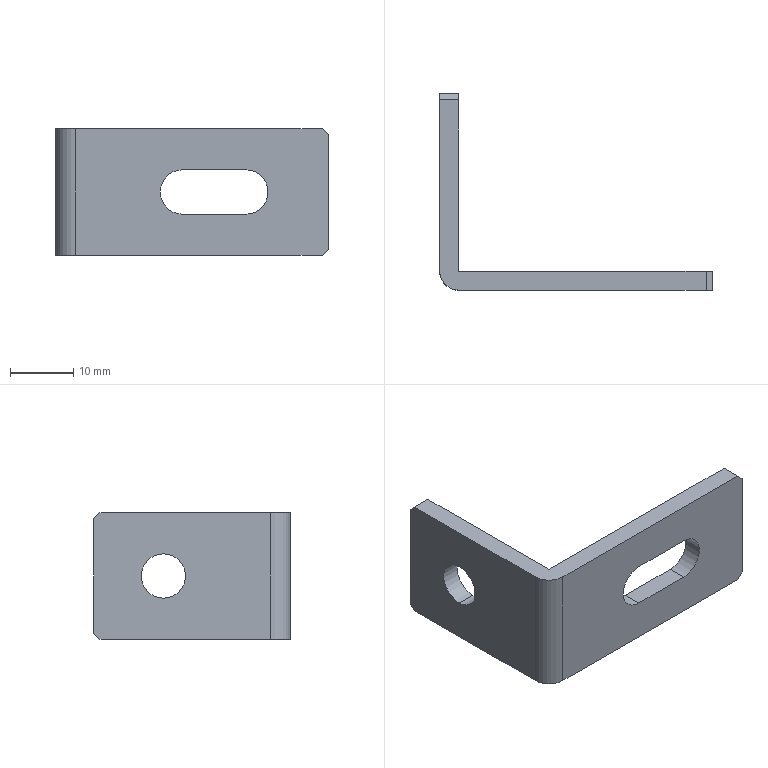Part | SolidWorks | features BaseBody 1 | 1 solid | 21 faces | box 43 x 31 x 20 mm | volume 3772 mm3 | plane 14 | cylinder 7 | commonest cylinder face diameters 7 x5 0.2 x1 6.2 x1
STEP:
#1=CARTESIAN_POINT('',(16.5,-31.,10.));
#2=VERTEX_POINT('',#1);
#3=CARTESIAN_POINT('',(20.,-31.,13.5));
#4=VERTEX_POINT('',#3);
#5=CARTESIAN_POINT('',(20.,-31.,10.));
#6=DIRECTION('',(0.,1.,0.));
#7=DIRECTION('',(-1.,0.,0.));
#8=AXIS2_PLACEMENT_3D('',#5,#6,#7);
#9=CIRCLE('',#8,3.5);
#10=EDGE_CURVE('',#2,#4,#9,.T.);
#11=ORIENTED_EDGE('',*,*,#10,.F.);
#12=CARTESIAN_POINT('',(16.5,-28.,10.));
#13=VERTEX_POINT('',#12);
#14=CARTESIAN_POINT('',(16.5,-31.,10.));
#15=DIRECTION('',(0.,1.,0.));
#16=VECTOR('',#15,1000.);
#17=LINE('',#14,#16);
#18=EDGE_CURVE('',#2,#13,#17,.T.);
#19=ORIENTED_EDGE('',*,*,#18,.T.);
#20=CARTESIAN_POINT('',(20.,-28.,13.5));
#21=VERTEX_POINT('',#20);
#22=CARTESIAN_POINT('',(20.,-28.,10.));
#23=DIRECTION('',(0.,1.,0.));
#24=DIRECTION('',(-1.,0.,0.));
#25=AXIS2_PLACEMENT_3D('',#22,#23,#24);
#26=CIRCLE('',#25,3.5);
#27=EDGE_CURVE('',#13,#21,#26,.T.);
#28=ORIENTED_EDGE('',*,*,#27,.T.);
#29=CARTESIAN_POINT('',(20.,-31.,13.5));
#30=DIRECTION('',(0.,-1.,0.));
#31=VECTOR('',#30,1000.);
#32=LINE('',#29,#31);
#33=EDGE_CURVE('',#21,#4,#32,.T.);
#34=ORIENTED_EDGE('',*,*,#33,.T.);
#35=EDGE_LOOP('',(#11,#19,#28,#34));
#36=FACE_OUTER_BOUND('',#35,.T.);
#37=CARTESIAN_POINT('',(20.,-31.,10.));
#38=DIRECTION('',(0.,1.,0.));
#39=DIRECTION('',(-1.,0.,0.));
#40=AXIS2_PLACEMENT_3D('',#37,#38,#39);
#41=CYLINDRICAL_SURFACE('',#40,3.5);
#42=ADVANCED_FACE('',(#36),#41,.F.);
#43=CARTESIAN_POINT('',(0.,-11.,13.5));
#44=VERTEX_POINT('',#43);
#45=CARTESIAN_POINT('',(0.,-11.,6.5));
#46=VERTEX_POINT('',#45);
#47=CARTESIAN_POINT('',(0.,-11.,10.));
#48=DIRECTION('',(1.,0.,0.));
#49=DIRECTION('',(0.,0.,-1.));
#50=AXIS2_PLACEMENT_3D('',#47,#48,#49);
#51=CIRCLE('',#50,3.5);
#52=EDGE_CURVE('',#44,#46,#51,.T.);
#53=ORIENTED_EDGE('',*,*,#52,.F.);
#54=CARTESIAN_POINT('',(3.,-11.,13.5));
#55=VERTEX_POINT('',#54);
#56=CARTESIAN_POINT('',(3.,-11.,13.5));
#57=DIRECTION('',(1.,0.,0.));
#58=VECTOR('',#57,1000.);
#59=LINE('',#56,#58);
#60=EDGE_CURVE('',#44,#55,#59,.T.);
#61=ORIENTED_EDGE('',*,*,#60,.T.);
#62=CARTESIAN_POINT('',(3.,-11.,6.5));
#63=VERTEX_POINT('',#62);
#64=CARTESIAN_POINT('',(3.,-11.,10.));
#65=DIRECTION('',(1.,0.,0.));
#66=DIRECTION('',(0.,0.,-1.));
#67=AXIS2_PLACEMENT_3D('',#64,#65,#66);
#68=CIRCLE('',#67,3.5);
#69=EDGE_CURVE('',#55,#63,#68,.T.);
#70=ORIENTED_EDGE('',*,*,#69,.T.);
#71=CARTESIAN_POINT('',(3.,-11.,6.5));
#72=DIRECTION('',(1.,0.,0.));
#73=VECTOR('',#72,1000.);
#74=LINE('',#71,#73);
#75=EDGE_CURVE('',#46,#63,#74,.T.);
#76=ORIENTED_EDGE('',*,*,#75,.F.);
#77=EDGE_LOOP('',(#53,#61,#70,#76));
#78=FACE_OUTER_BOUND('',#77,.T.);
#79=CARTESIAN_POINT('',(3.,-11.,10.));
#80=DIRECTION('',(1.,0.,0.));
#81=DIRECTION('',(0.,0.,-1.));
#82=AXIS2_PLACEMENT_3D('',#79,#80,#81);
#83=CYLINDRICAL_SURFACE('',#82,3.5);
#84=ADVANCED_FACE('',(#78),#83,.F.);
#85=CARTESIAN_POINT('',(43.,-28.,1.));
#86=VERTEX_POINT('',#85);
#87=CARTESIAN_POINT('',(42.,-28.,0.));
#88=VERTEX_POINT('',#87);
#89=CARTESIAN_POINT('',(42.,-28.,0.));
#90=DIRECTION('',(-0.7071,0.,-0.7071));
#91=VECTOR('',#90,1000.);
#92=LINE('',#89,#91);
#93=EDGE_CURVE('',#86,#88,#92,.T.);
#94=ORIENTED_EDGE('',*,*,#93,.T.);
#95=CARTESIAN_POINT('',(3.1,-28.,0.));
#96=VERTEX_POINT('',#95);
#97=CARTESIAN_POINT('',(43.,-28.,0.));
#98=DIRECTION('',(1.,0.,0.));
#99=VECTOR('',#98,1000.);
#100=LINE('',#97,#99);
#101=EDGE_CURVE('',#96,#88,#100,.T.);
#102=ORIENTED_EDGE('',*,*,#101,.F.);
#103=CARTESIAN_POINT('',(3.1,-28.,20.));
#104=VERTEX_POINT('',#103);
#105=CARTESIAN_POINT('',(3.1,-28.,20.));
#106=DIRECTION('',(0.,0.,-1.));
#107=VECTOR('',#106,1000.);
#108=LINE('',#105,#107);
#109=EDGE_CURVE('',#104,#96,#108,.T.);
#110=ORIENTED_EDGE('',*,*,#109,.F.);
#111=CARTESIAN_POINT('',(42.,-28.,20.));
#112=VERTEX_POINT('',#111);
#113=CARTESIAN_POINT('',(43.,-28.,20.));
#114=DIRECTION('',(-1.,0.,0.));
#115=VECTOR('',#114,1000.);
#116=LINE('',#113,#115);
#117=EDGE_CURVE('',#112,#104,#116,.T.);
#118=ORIENTED_EDGE('',*,*,#117,.F.);
#119=CARTESIAN_POINT('',(43.,-28.,19.));
#120=VERTEX_POINT('',#119);
#121=CARTESIAN_POINT('',(43.,-28.,19.));
#122=DIRECTION('',(-0.7071,0.,0.7071));
#123=VECTOR('',#122,1000.);
#124=LINE('',#121,#123);
#125=EDGE_CURVE('',#120,#112,#124,.T.);
#126=ORIENTED_EDGE('',*,*,#125,.F.);
#127=CARTESIAN_POINT('',(43.,-28.,20.));
#128=DIRECTION('',(0.,0.,1.));
#129=VECTOR('',#128,1000.);
#130=LINE('',#127,#129);
#131=EDGE_CURVE('',#86,#120,#130,.T.);
#132=ORIENTED_EDGE('',*,*,#131,.F.);
#133=EDGE_LOOP('',(#94,#102,#110,#118,#126,#132));
#134=FACE_OUTER_BOUND('',#133,.T.);
#135=CARTESIAN_POINT('',(30.,-28.,13.5));
#136=VERTEX_POINT('',#135);
#137=CARTESIAN_POINT('',(43.,-28.,13.5));
#138=DIRECTION('',(1.,0.,0.));
#139=VECTOR('',#138,1000.);
#140=LINE('',#137,#139);
#141=EDGE_CURVE('',#21,#136,#140,.T.);
#142=ORIENTED_EDGE('',*,*,#141,.F.);
#143=ORIENTED_EDGE('',*,*,#27,.F.);
#144=CARTESIAN_POINT('',(20.,-28.,6.5));
#145=VERTEX_POINT('',#144);
#146=CARTESIAN_POINT('',(20.,-28.,10.));
#147=DIRECTION('',(0.,1.,0.));
#148=DIRECTION('',(-1.,0.,0.));
#149=AXIS2_PLACEMENT_3D('',#146,#147,#148);
#150=CIRCLE('',#149,3.5);
#151=EDGE_CURVE('',#145,#13,#150,.T.);
#152=ORIENTED_EDGE('',*,*,#151,.F.);
#153=CARTESIAN_POINT('',(30.,-28.,6.5));
#154=VERTEX_POINT('',#153);
#155=CARTESIAN_POINT('',(43.,-28.,6.5));
#156=DIRECTION('',(-1.,0.,0.));
#157=VECTOR('',#156,1000.);
#158=LINE('',#155,#157);
#159=EDGE_CURVE('',#154,#145,#158,.T.);
#160=ORIENTED_EDGE('',*,*,#159,.F.);
#161=CARTESIAN_POINT('',(30.,-28.,10.));
#162=DIRECTION('',(0.,1.,0.));
#163=DIRECTION('',(-1.,0.,0.));
#164=AXIS2_PLACEMENT_3D('',#161,#162,#163);
#165=CIRCLE('',#164,3.5);
#166=EDGE_CURVE('',#136,#154,#165,.T.);
#167=ORIENTED_EDGE('',*,*,#166,.F.);
#168=EDGE_LOOP('',(#142,#143,#152,#160,#167));
#169=FACE_BOUND('',#168,.T.);
#170=CARTESIAN_POINT('',(43.,-28.,20.));
#171=DIRECTION('',(0.,-1.,0.));
#172=DIRECTION('',(1.,0.,0.));
#173=AXIS2_PLACEMENT_3D('',#170,#171,#172);
#174=PLANE('',#173);
#175=ADVANCED_FACE('',(#134,#169),#174,.F.);
#176=ORIENTED_EDGE('',*,*,#131,.T.);
#177=CARTESIAN_POINT('',(43.,-31.,19.));
#178=VERTEX_POINT('',#177);
#179=CARTESIAN_POINT('',(43.,-28.,19.));
#180=DIRECTION('',(0.,-1.,0.));
#181=VECTOR('',#180,1000.);
#182=LINE('',#179,#181);
#183=EDGE_CURVE('',#120,#178,#182,.T.);
#184=ORIENTED_EDGE('',*,*,#183,.T.);
#185=CARTESIAN_POINT('',(43.,-31.,1.));
#186=VERTEX_POINT('',#185);
#187=CARTESIAN_POINT('',(43.,-31.,20.));
#188=DIRECTION('',(0.,0.,-1.));
#189=VECTOR('',#188,1000.);
#190=LINE('',#187,#189);
#191=EDGE_CURVE('',#178,#186,#190,.T.);
#192=ORIENTED_EDGE('',*,*,#191,.T.);
#193=CARTESIAN_POINT('',(43.,-28.,1.));
#194=DIRECTION('',(0.,1.,0.));
#195=VECTOR('',#194,1000.);
#196=LINE('',#193,#195);
#197=EDGE_CURVE('',#186,#86,#196,.T.);
#198=ORIENTED_EDGE('',*,*,#197,.T.);
#199=EDGE_LOOP('',(#176,#184,#192,#198));
#200=FACE_OUTER_BOUND('',#199,.T.);
#201=CARTESIAN_POINT('',(43.,-28.,20.));
#202=DIRECTION('',(1.,0.,0.));
#203=DIRECTION('',(0.,0.,-1.));
#204=AXIS2_PLACEMENT_3D('',#201,#202,#203);
#205=PLANE('',#204);
#206=ADVANCED_FACE('',(#200),#205,.T.);
#207=CARTESIAN_POINT('',(42.,-31.,0.));
#208=VERTEX_POINT('',#207);
#209=CARTESIAN_POINT('',(3.1,-31.,0.));
#210=VERTEX_POINT('',#209);
#211=CARTESIAN_POINT('',(3.,-31.,0.));
#212=DIRECTION('',(-1.,0.,0.));
#213=VECTOR('',#212,1000.);
#214=LINE('',#211,#213);
#215=EDGE_CURVE('',#208,#210,#214,.T.);
#216=ORIENTED_EDGE('',*,*,#215,.T.);
#217=CARTESIAN_POINT('',(0.,-27.9,0.));
#218=VERTEX_POINT('',#217);
#219=CARTESIAN_POINT('',(3.1,-27.9,0.));
#220=DIRECTION('',(0.,0.,-1.));
#221=DIRECTION('',(-1.,0.,0.));
#222=AXIS2_PLACEMENT_3D('',#219,#220,#221);
#223=CIRCLE('',#222,3.1);
#224=EDGE_CURVE('',#210,#218,#223,.T.);
#225=ORIENTED_EDGE('',*,*,#224,.T.);
#226=CARTESIAN_POINT('',(0.,-1.,0.));
#227=VERTEX_POINT('',#226);
#228=CARTESIAN_POINT('',(0.,-27.9,0.));
#229=DIRECTION('',(0.,1.,0.));
#230=VECTOR('',#229,1000.);
#231=LINE('',#228,#230);
#232=EDGE_CURVE('',#218,#227,#231,.T.);
#233=ORIENTED_EDGE('',*,*,#232,.T.);
#234=CARTESIAN_POINT('',(3.,-1.,0.));
#235=VERTEX_POINT('',#234);
#236=CARTESIAN_POINT('',(3.1,-1.,0.));
#237=DIRECTION('',(1.,0.,0.));
#238=VECTOR('',#237,1000.);
#239=LINE('',#236,#238);
#240=EDGE_CURVE('',#227,#235,#239,.T.);
#241=ORIENTED_EDGE('',*,*,#240,.T.);
#242=CARTESIAN_POINT('',(3.,-27.9,0.));
#243=VERTEX_POINT('',#242);
#244=CARTESIAN_POINT('',(3.,0.,0.));
#245=DIRECTION('',(0.,-1.,0.));
#246=VECTOR('',#245,1000.);
#247=LINE('',#244,#246);
#248=EDGE_CURVE('',#235,#243,#247,.T.);
#249=ORIENTED_EDGE('',*,*,#248,.T.);
#250=CARTESIAN_POINT('',(3.1,-27.9,0.));
#251=DIRECTION('',(0.,0.,1.));
#252=DIRECTION('',(-1.,0.,0.));
#253=AXIS2_PLACEMENT_3D('',#250,#251,#252);
#254=CIRCLE('',#253,0.1);
#255=EDGE_CURVE('',#243,#96,#254,.T.);
#256=ORIENTED_EDGE('',*,*,#255,.T.);
#257=ORIENTED_EDGE('',*,*,#101,.T.);
#258=CARTESIAN_POINT('',(42.,-27.9,0.));
#259=DIRECTION('',(0.,-1.,0.));
#260=VECTOR('',#259,1000.);
#261=LINE('',#258,#260);
#262=EDGE_CURVE('',#88,#208,#261,.T.);
#263=ORIENTED_EDGE('',*,*,#262,.T.);
#264=EDGE_LOOP('',(#216,#225,#233,#241,#249,#256,#257,#263));
#265=FACE_OUTER_BOUND('',#264,.T.);
#266=CARTESIAN_POINT('',(3.,-27.9,0.));
#267=DIRECTION('',(0.,0.,-1.));
#268=DIRECTION('',(-1.,0.,0.));
#269=AXIS2_PLACEMENT_3D('',#266,#267,#268);
#270=PLANE('',#269);
#271=ADVANCED_FACE('',(#265),#270,.T.);
#272=CARTESIAN_POINT('',(3.,-27.9,20.));
#273=VERTEX_POINT('',#272);
#274=CARTESIAN_POINT('',(3.,-27.9,20.));
#275=DIRECTION('',(0.,0.,-1.));
#276=VECTOR('',#275,1000.);
#277=LINE('',#274,#276);
#278=EDGE_CURVE('',#273,#243,#277,.T.);
#279=ORIENTED_EDGE('',*,*,#278,.F.);
#280=CARTESIAN_POINT('',(3.1,-27.9,20.));
#281=DIRECTION('',(0.,0.,-1.));
#282=DIRECTION('',(-1.,0.,0.));
#283=AXIS2_PLACEMENT_3D('',#280,#281,#282);
#284=CIRCLE('',#283,0.1);
#285=EDGE_CURVE('',#104,#273,#284,.T.);
#286=ORIENTED_EDGE('',*,*,#285,.F.);
#287=ORIENTED_EDGE('',*,*,#109,.T.);
#288=ORIENTED_EDGE('',*,*,#255,.F.);
#289=EDGE_LOOP('',(#279,#286,#287,#288));
#290=FACE_OUTER_BOUND('',#289,.T.);
#291=CARTESIAN_POINT('',(3.1,-27.9,20.));
#292=DIRECTION('',(0.,0.,-1.));
#293=DIRECTION('',(-1.,0.,0.));
#294=AXIS2_PLACEMENT_3D('',#291,#292,#293);
#295=CYLINDRICAL_SURFACE('',#294,0.1);
#296=ADVANCED_FACE('',(#290),#295,.F.);
#297=CARTESIAN_POINT('',(42.,-31.,20.));
#298=VERTEX_POINT('',#297);
#299=CARTESIAN_POINT('',(42.,-27.9,20.));
#300=DIRECTION('',(0.,-1.,0.));
#301=VECTOR('',#300,1000.);
#302=LINE('',#299,#301);
#303=EDGE_CURVE('',#112,#298,#302,.T.);
#304=ORIENTED_EDGE('',*,*,#303,.F.);
#305=ORIENTED_EDGE('',*,*,#117,.T.);
#306=ORIENTED_EDGE('',*,*,#285,.T.);
#307=CARTESIAN_POINT('',(3.,-1.,20.));
#308=VERTEX_POINT('',#307);
#309=CARTESIAN_POINT('',(3.,0.,20.));
#310=DIRECTION('',(0.,1.,0.));
#311=VECTOR('',#310,1000.);
#312=LINE('',#309,#311);
#313=EDGE_CURVE('',#273,#308,#312,.T.);
#314=ORIENTED_EDGE('',*,*,#313,.T.);
#315=CARTESIAN_POINT('',(0.,-1.,20.));
#316=VERTEX_POINT('',#315);
#317=CARTESIAN_POINT('',(3.1,-1.,20.));
#318=DIRECTION('',(-1.,0.,0.));
#319=VECTOR('',#318,1000.);
#320=LINE('',#317,#319);
#321=EDGE_CURVE('',#308,#316,#320,.T.);
#322=ORIENTED_EDGE('',*,*,#321,.T.);
#323=CARTESIAN_POINT('',(0.,-27.9,20.));
#324=VERTEX_POINT('',#323);
#325=CARTESIAN_POINT('',(0.,-28.,20.));
#326=DIRECTION('',(0.,-1.,0.));
#327=VECTOR('',#326,1000.);
#328=LINE('',#325,#327);
#329=EDGE_CURVE('',#316,#324,#328,.T.);
#330=ORIENTED_EDGE('',*,*,#329,.T.);
#331=CARTESIAN_POINT('',(3.1,-31.,20.));
#332=VERTEX_POINT('',#331);
#333=CARTESIAN_POINT('',(3.1,-27.9,20.));
#334=DIRECTION('',(0.,0.,1.));
#335=DIRECTION('',(-1.,0.,0.));
#336=AXIS2_PLACEMENT_3D('',#333,#334,#335);
#337=CIRCLE('',#336,3.1);
#338=EDGE_CURVE('',#324,#332,#337,.T.);
#339=ORIENTED_EDGE('',*,*,#338,.T.);
#340=CARTESIAN_POINT('',(3.1,-31.,20.));
#341=DIRECTION('',(-1.,0.,0.));
#342=VECTOR('',#341,1000.);
#343=LINE('',#340,#342);
#344=EDGE_CURVE('',#298,#332,#343,.T.);
#345=ORIENTED_EDGE('',*,*,#344,.F.);
#346=EDGE_LOOP('',(#304,#305,#306,#314,#322,#330,#339,#345));
#347=FACE_OUTER_BOUND('',#346,.T.);
#348=CARTESIAN_POINT('',(3.1,-27.9,20.));
#349=DIRECTION('',(0.,0.,-1.));
#350=DIRECTION('',(-1.,0.,0.));
#351=AXIS2_PLACEMENT_3D('',#348,#349,#350);
#352=PLANE('',#351);
#353=ADVANCED_FACE('',(#347),#352,.F.);
#354=CARTESIAN_POINT('',(30.,-31.,13.5));
#355=VERTEX_POINT('',#354);
#356=CARTESIAN_POINT('',(30.,-31.,13.5));
#357=DIRECTION('',(0.,1.,0.));
#358=VECTOR('',#357,1000.);
#359=LINE('',#356,#358);
#360=EDGE_CURVE('',#355,#136,#359,.T.);
#361=ORIENTED_EDGE('',*,*,#360,.F.);
#362=CARTESIAN_POINT('',(20.,-31.,13.5));
#363=DIRECTION('',(1.,0.,0.));
#364=VECTOR('',#363,1000.);
#365=LINE('',#362,#364);
#366=EDGE_CURVE('',#4,#355,#365,.T.);
#367=ORIENTED_EDGE('',*,*,#366,.F.);
#368=ORIENTED_EDGE('',*,*,#33,.F.);
#369=ORIENTED_EDGE('',*,*,#141,.T.);
#370=EDGE_LOOP('',(#361,#367,#368,#369));
#371=FACE_OUTER_BOUND('',#370,.T.);
#372=CARTESIAN_POINT('',(20.,-31.,13.5));
#373=DIRECTION('',(0.,0.,1.));
#374=DIRECTION('',(1.,0.,0.));
#375=AXIS2_PLACEMENT_3D('',#372,#373,#374);
#376=PLANE('',#375);
#377=ADVANCED_FACE('',(#371),#376,.F.);
#378=ORIENTED_EDGE('',*,*,#18,.F.);
#379=CARTESIAN_POINT('',(20.,-31.,6.5));
#380=VERTEX_POINT('',#379);
#381=CARTESIAN_POINT('',(20.,-31.,10.));
#382=DIRECTION('',(0.,1.,0.));
#383=DIRECTION('',(-1.,0.,0.));
#384=AXIS2_PLACEMENT_3D('',#381,#382,#383);
#385=CIRCLE('',#384,3.5);
#386=EDGE_CURVE('',#380,#2,#385,.T.);
#387=ORIENTED_EDGE('',*,*,#386,.F.);
#388=CARTESIAN_POINT('',(20.,-31.,6.5));
#389=DIRECTION('',(0.,-1.,0.));
#390=VECTOR('',#389,1000.);
#391=LINE('',#388,#390);
#392=EDGE_CURVE('',#145,#380,#391,.T.);
#393=ORIENTED_EDGE('',*,*,#392,.F.);
#394=ORIENTED_EDGE('',*,*,#151,.T.);
#395=EDGE_LOOP('',(#378,#387,#393,#394));
#396=FACE_OUTER_BOUND('',#395,.T.);
#397=CARTESIAN_POINT('',(20.,-31.,10.));
#398=DIRECTION('',(0.,1.,0.));
#399=DIRECTION('',(-1.,0.,0.));
#400=AXIS2_PLACEMENT_3D('',#397,#398,#399);
#401=CYLINDRICAL_SURFACE('',#400,3.5);
#402=ADVANCED_FACE('',(#396),#401,.F.);
#403=ORIENTED_EDGE('',*,*,#392,.T.);
#404=CARTESIAN_POINT('',(30.,-31.,6.5));
#405=VERTEX_POINT('',#404);
#406=CARTESIAN_POINT('',(20.,-31.,6.5));
#407=DIRECTION('',(-1.,0.,0.));
#408=VECTOR('',#407,1000.);
#409=LINE('',#406,#408);
#410=EDGE_CURVE('',#405,#380,#409,.T.);
#411=ORIENTED_EDGE('',*,*,#410,.F.);
#412=CARTESIAN_POINT('',(30.,-31.,6.5));
#413=DIRECTION('',(0.,-1.,0.));
#414=VECTOR('',#413,1000.);
#415=LINE('',#412,#414);
#416=EDGE_CURVE('',#154,#405,#415,.T.);
#417=ORIENTED_EDGE('',*,*,#416,.F.);
#418=ORIENTED_EDGE('',*,*,#159,.T.);
#419=EDGE_LOOP('',(#403,#411,#417,#418));
#420=FACE_OUTER_BOUND('',#419,.T.);
#421=CARTESIAN_POINT('',(20.,-31.,6.5));
#422=DIRECTION('',(0.,0.,-1.));
#423=DIRECTION('',(-1.,0.,0.));
#424=AXIS2_PLACEMENT_3D('',#421,#422,#423);
#425=PLANE('',#424);
#426=ADVANCED_FACE('',(#420),#425,.F.);
#427=ORIENTED_EDGE('',*,*,#416,.T.);
#428=CARTESIAN_POINT('',(30.,-31.,10.));
#429=DIRECTION('',(0.,1.,0.));
#430=DIRECTION('',(-1.,0.,0.));
#431=AXIS2_PLACEMENT_3D('',#428,#429,#430);
#432=CIRCLE('',#431,3.5);
#433=EDGE_CURVE('',#355,#405,#432,.T.);
#434=ORIENTED_EDGE('',*,*,#433,.F.);
#435=ORIENTED_EDGE('',*,*,#360,.T.);
#436=ORIENTED_EDGE('',*,*,#166,.T.);
#437=EDGE_LOOP('',(#427,#434,#435,#436));
#438=FACE_OUTER_BOUND('',#437,.T.);
#439=CARTESIAN_POINT('',(30.,-31.,10.));
#440=DIRECTION('',(0.,1.,0.));
#441=DIRECTION('',(-1.,0.,0.));
#442=AXIS2_PLACEMENT_3D('',#439,#440,#441);
#443=CYLINDRICAL_SURFACE('',#442,3.5);
#444=ADVANCED_FACE('',(#438),#443,.F.);
#445=CARTESIAN_POINT('',(43.,-31.,19.));
#446=DIRECTION('',(0.7071,0.,-0.7071));
#447=VECTOR('',#446,1000.);
#448=LINE('',#445,#447);
#449=EDGE_CURVE('',#298,#178,#448,.T.);
#450=ORIENTED_EDGE('',*,*,#449,.T.);
#451=ORIENTED_EDGE('',*,*,#183,.F.);
#452=ORIENTED_EDGE('',*,*,#125,.T.);
#453=ORIENTED_EDGE('',*,*,#303,.T.);
#454=EDGE_LOOP('',(#450,#451,#452,#453));
#455=FACE_OUTER_BOUND('',#454,.T.);
#456=CARTESIAN_POINT('',(43.,-28.,19.));
#457=DIRECTION('',(0.7071,0.,0.7071));
#458=DIRECTION('',(0.7071,0.,-0.7071));
#459=AXIS2_PLACEMENT_3D('',#456,#457,#458);
#460=PLANE('',#459);
#461=ADVANCED_FACE('',(#455),#460,.T.);
#462=ORIENTED_EDGE('',*,*,#197,.F.);
#463=CARTESIAN_POINT('',(42.,-31.,0.));
#464=DIRECTION('',(0.7071,0.,0.7071));
#465=VECTOR('',#464,1000.);
#466=LINE('',#463,#465);
#467=EDGE_CURVE('',#208,#186,#466,.T.);
#468=ORIENTED_EDGE('',*,*,#467,.F.);
#469=ORIENTED_EDGE('',*,*,#262,.F.);
#470=ORIENTED_EDGE('',*,*,#93,.F.);
#471=EDGE_LOOP('',(#462,#468,#469,#470));
#472=FACE_OUTER_BOUND('',#471,.T.);
#473=CARTESIAN_POINT('',(42.,-27.9,0.));
#474=DIRECTION('',(-0.7071,0.,0.7071));
#475=DIRECTION('',(0.7071,0.,0.7071));
#476=AXIS2_PLACEMENT_3D('',#473,#474,#475);
#477=PLANE('',#476);
#478=ADVANCED_FACE('',(#472),#477,.F.);
#479=ORIENTED_EDGE('',*,*,#344,.T.);
#480=CARTESIAN_POINT('',(3.1,-31.,20.));
#481=DIRECTION('',(0.,0.,-1.));
#482=VECTOR('',#481,1000.);
#483=LINE('',#480,#482);
#484=EDGE_CURVE('',#332,#210,#483,.T.);
#485=ORIENTED_EDGE('',*,*,#484,.T.);
#486=ORIENTED_EDGE('',*,*,#215,.F.);
#487=ORIENTED_EDGE('',*,*,#467,.T.);
#488=ORIENTED_EDGE('',*,*,#191,.F.);
#489=ORIENTED_EDGE('',*,*,#449,.F.);
#490=EDGE_LOOP('',(#479,#485,#486,#487,#488,#489));
#491=FACE_OUTER_BOUND('',#490,.T.);
#492=ORIENTED_EDGE('',*,*,#433,.T.);
#493=ORIENTED_EDGE('',*,*,#410,.T.);
#494=ORIENTED_EDGE('',*,*,#386,.T.);
#495=ORIENTED_EDGE('',*,*,#10,.T.);
#496=ORIENTED_EDGE('',*,*,#366,.T.);
#497=EDGE_LOOP('',(#492,#493,#494,#495,#496));
#498=FACE_BOUND('',#497,.T.);
#499=CARTESIAN_POINT('',(43.,-31.,20.));
#500=DIRECTION('',(0.,-1.,0.));
#501=DIRECTION('',(1.,0.,0.));
#502=AXIS2_PLACEMENT_3D('',#499,#500,#501);
#503=PLANE('',#502);
#504=ADVANCED_FACE('',(#491,#498),#503,.T.);
#505=CARTESIAN_POINT('',(3.,0.,1.));
#506=VERTEX_POINT('',#505);
#507=CARTESIAN_POINT('',(3.,-1.,0.));
#508=DIRECTION('',(0.,0.7071,0.7071));
#509=VECTOR('',#508,1000.);
#510=LINE('',#507,#509);
#511=EDGE_CURVE('',#235,#506,#510,.T.);
#512=ORIENTED_EDGE('',*,*,#511,.T.);
#513=CARTESIAN_POINT('',(3.,0.,19.));
#514=VERTEX_POINT('',#513);
#515=CARTESIAN_POINT('',(3.,0.,20.));
#516=DIRECTION('',(0.,0.,-1.));
#517=VECTOR('',#516,1000.);
#518=LINE('',#515,#517);
#519=EDGE_CURVE('',#514,#506,#518,.T.);
#520=ORIENTED_EDGE('',*,*,#519,.F.);
#521=CARTESIAN_POINT('',(3.,0.,19.));
#522=DIRECTION('',(0.,-0.7071,0.7071));
#523=VECTOR('',#522,1000.);
#524=LINE('',#521,#523);
#525=EDGE_CURVE('',#514,#308,#524,.T.);
#526=ORIENTED_EDGE('',*,*,#525,.T.);
#527=ORIENTED_EDGE('',*,*,#313,.F.);
#528=ORIENTED_EDGE('',*,*,#278,.T.);
#529=ORIENTED_EDGE('',*,*,#248,.F.);
#530=EDGE_LOOP('',(#512,#520,#526,#527,#528,#529));
#531=FACE_OUTER_BOUND('',#530,.T.);
#532=CARTESIAN_POINT('',(3.,-11.,10.));
#533=DIRECTION('',(1.,0.,0.));
#534=DIRECTION('',(0.,0.,-1.));
#535=AXIS2_PLACEMENT_3D('',#532,#533,#534);
#536=CIRCLE('',#535,3.5);
#537=EDGE_CURVE('',#63,#55,#536,.T.);
#538=ORIENTED_EDGE('',*,*,#537,.F.);
#539=ORIENTED_EDGE('',*,*,#69,.F.);
#540=EDGE_LOOP('',(#538,#539));
#541=FACE_BOUND('',#540,.T.);
#542=CARTESIAN_POINT('',(3.,0.,20.));
#543=DIRECTION('',(-1.,0.,0.));
#544=DIRECTION('',(0.,-1.,0.));
#545=AXIS2_PLACEMENT_3D('',#542,#543,#544);
#546=PLANE('',#545);
#547=ADVANCED_FACE('',(#531,#541),#546,.F.);
#548=ORIENTED_EDGE('',*,*,#338,.F.);
#549=CARTESIAN_POINT('',(0.,-27.9,20.));
#550=DIRECTION('',(0.,0.,-1.));
#551=VECTOR('',#550,1000.);
#552=LINE('',#549,#551);
#553=EDGE_CURVE('',#324,#218,#552,.T.);
#554=ORIENTED_EDGE('',*,*,#553,.T.);
#555=ORIENTED_EDGE('',*,*,#224,.F.);
#556=ORIENTED_EDGE('',*,*,#484,.F.);
#557=EDGE_LOOP('',(#548,#554,#555,#556));
#558=FACE_OUTER_BOUND('',#557,.T.);
#559=CARTESIAN_POINT('',(3.1,-27.9,20.));
#560=DIRECTION('',(0.,0.,-1.));
#561=DIRECTION('',(-1.,0.,0.));
#562=AXIS2_PLACEMENT_3D('',#559,#560,#561);
#563=CYLINDRICAL_SURFACE('',#562,3.1);
#564=ADVANCED_FACE('',(#558),#563,.T.);
#565=CARTESIAN_POINT('',(0.,0.,1.));
#566=VERTEX_POINT('',#565);
#567=CARTESIAN_POINT('',(0.,0.,19.));
#568=VERTEX_POINT('',#567);
#569=CARTESIAN_POINT('',(0.,0.,20.));
#570=DIRECTION('',(0.,0.,1.));
#571=VECTOR('',#570,1000.);
#572=LINE('',#569,#571);
#573=EDGE_CURVE('',#566,#568,#572,.T.);
#574=ORIENTED_EDGE('',*,*,#573,.T.);
#575=CARTESIAN_POINT('',(0.,0.,19.));
#576=DIRECTION('',(1.,0.,0.));
#577=VECTOR('',#576,1000.);
#578=LINE('',#575,#577);
#579=EDGE_CURVE('',#568,#514,#578,.T.);
#580=ORIENTED_EDGE('',*,*,#579,.T.);
#581=ORIENTED_EDGE('',*,*,#519,.T.);
#582=CARTESIAN_POINT('',(0.,0.,1.));
#583=DIRECTION('',(-1.,0.,0.));
#584=VECTOR('',#583,1000.);
#585=LINE('',#582,#584);
#586=EDGE_CURVE('',#506,#566,#585,.T.);
#587=ORIENTED_EDGE('',*,*,#586,.T.);
#588=EDGE_LOOP('',(#574,#580,#581,#587));
#589=FACE_OUTER_BOUND('',#588,.T.);
#590=CARTESIAN_POINT('',(0.,0.,20.));
#591=DIRECTION('',(0.,1.,0.));
#592=DIRECTION('',(-1.,0.,0.));
#593=AXIS2_PLACEMENT_3D('',#590,#591,#592);
#594=PLANE('',#593);
#595=ADVANCED_FACE('',(#589),#594,.T.);
#596=ORIENTED_EDGE('',*,*,#60,.F.);
#597=CARTESIAN_POINT('',(0.,-11.,10.));
#598=DIRECTION('',(1.,0.,0.));
#599=DIRECTION('',(0.,0.,-1.));
#600=AXIS2_PLACEMENT_3D('',#597,#598,#599);
#601=CIRCLE('',#600,3.5);
#602=EDGE_CURVE('',#46,#44,#601,.T.);
#603=ORIENTED_EDGE('',*,*,#602,.F.);
#604=ORIENTED_EDGE('',*,*,#75,.T.);
#605=ORIENTED_EDGE('',*,*,#537,.T.);
#606=EDGE_LOOP('',(#596,#603,#604,#605));
#607=FACE_OUTER_BOUND('',#606,.T.);
#608=CARTESIAN_POINT('',(3.,-11.,10.));
#609=DIRECTION('',(1.,0.,0.));
#610=DIRECTION('',(0.,0.,-1.));
#611=AXIS2_PLACEMENT_3D('',#608,#609,#610);
#612=CYLINDRICAL_SURFACE('',#611,3.5);
#613=ADVANCED_FACE('',(#607),#612,.F.);
#614=ORIENTED_EDGE('',*,*,#329,.F.);
#615=CARTESIAN_POINT('',(0.,-1.,20.));
#616=DIRECTION('',(0.,0.7071,-0.7071));
#617=VECTOR('',#616,1000.);
#618=LINE('',#615,#617);
#619=EDGE_CURVE('',#316,#568,#618,.T.);
#620=ORIENTED_EDGE('',*,*,#619,.T.);
#621=ORIENTED_EDGE('',*,*,#573,.F.);
#622=CARTESIAN_POINT('',(0.,0.,1.));
#623=DIRECTION('',(0.,-0.7071,-0.7071));
#624=VECTOR('',#623,1000.);
#625=LINE('',#622,#624);
#626=EDGE_CURVE('',#566,#227,#625,.T.);
#627=ORIENTED_EDGE('',*,*,#626,.T.);
#628=ORIENTED_EDGE('',*,*,#232,.F.);
#629=ORIENTED_EDGE('',*,*,#553,.F.);
#630=EDGE_LOOP('',(#614,#620,#621,#627,#628,#629));
#631=FACE_OUTER_BOUND('',#630,.T.);
#632=ORIENTED_EDGE('',*,*,#602,.T.);
#633=ORIENTED_EDGE('',*,*,#52,.T.);
#634=EDGE_LOOP('',(#632,#633));
#635=FACE_BOUND('',#634,.T.);
#636=CARTESIAN_POINT('',(0.,0.,20.));
#637=DIRECTION('',(-1.,0.,0.));
#638=DIRECTION('',(0.,-1.,0.));
#639=AXIS2_PLACEMENT_3D('',#636,#637,#638);
#640=PLANE('',#639);
#641=ADVANCED_FACE('',(#631,#635),#640,.T.);
#642=ORIENTED_EDGE('',*,*,#586,.F.);
#643=ORIENTED_EDGE('',*,*,#511,.F.);
#644=ORIENTED_EDGE('',*,*,#240,.F.);
#645=ORIENTED_EDGE('',*,*,#626,.F.);
#646=EDGE_LOOP('',(#642,#643,#644,#645));
#647=FACE_OUTER_BOUND('',#646,.T.);
#648=CARTESIAN_POINT('',(3.1,-1.,0.));
#649=DIRECTION('',(0.,-0.7071,0.7071));
#650=DIRECTION('',(0.,-0.7071,-0.7071));
#651=AXIS2_PLACEMENT_3D('',#648,#649,#650);
#652=PLANE('',#651);
#653=ADVANCED_FACE('',(#647),#652,.F.);
#654=ORIENTED_EDGE('',*,*,#321,.F.);
#655=ORIENTED_EDGE('',*,*,#525,.F.);
#656=ORIENTED_EDGE('',*,*,#579,.F.);
#657=ORIENTED_EDGE('',*,*,#619,.F.);
#658=EDGE_LOOP('',(#654,#655,#656,#657));
#659=FACE_OUTER_BOUND('',#658,.T.);
#660=CARTESIAN_POINT('',(0.,0.,19.));
#661=DIRECTION('',(0.,-0.7071,-0.7071));
#662=DIRECTION('',(0.,0.7071,-0.7071));
#663=AXIS2_PLACEMENT_3D('',#660,#661,#662);
#664=PLANE('',#663);
#665=ADVANCED_FACE('',(#659),#664,.F.);
#666=CLOSED_SHELL('',(#42,#84,#175,#206,#271,#296,#353,#377,#402,#426,#444,#461,#478,#504,#547,#564,#595,#613,#641,#653,#665));
#667=MANIFOLD_SOLID_BREP('',#666);
#668=CARTESIAN_POINT('',(0.,0.,0.));
#669=DIRECTION('',(0.,0.,1.));
#670=DIRECTION('',(1.,0.,0.));
#671=AXIS2_PLACEMENT_3D('',#668,#669,#670);
#672=(LENGTH_UNIT()NAMED_UNIT(*)SI_UNIT(.MILLI.,.METRE.));
#673=UNCERTAINTY_MEASURE_WITH_UNIT(LENGTH_MEASURE(0.00001),#672,'','');
#674=(NAMED_UNIT(*)PLANE_ANGLE_UNIT()SI_UNIT($,.RADIAN.));
#675=(NAMED_UNIT(*)SI_UNIT($,.STERADIAN.)SOLID_ANGLE_UNIT());
#676=(GEOMETRIC_REPRESENTATION_CONTEXT(3)GLOBAL_UNCERTAINTY_ASSIGNED_CONTEXT((#673))GLOBAL_UNIT_ASSIGNED_CONTEXT((#672,#674,#675))REPRESENTATION_CONTEXT('',''));
#677=ADVANCED_BREP_SHAPE_REPRESENTATION('',(#667,#671),#676);